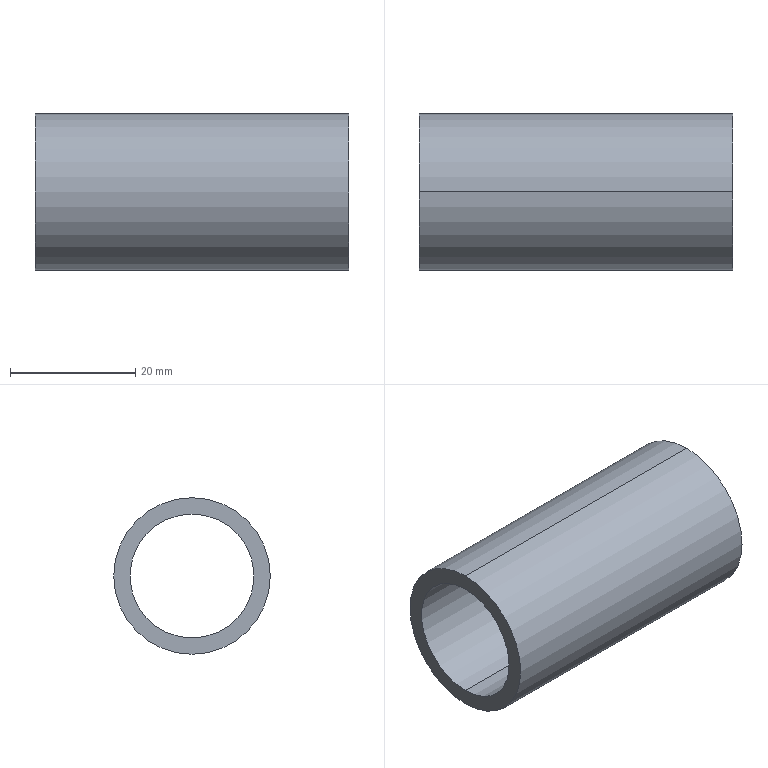Part | STEP file | FUF25-70-A-8 | 1 solid | 6 faces | box 50 x 25 x 25 mm | volume 9148 mm3 | cylinder 4 | plane 2 | commonest cylinder face diameters 19.8 x2 25 x2
STEP:
#1=CARTESIAN_POINT('',(0.,0.,0.));
#2=DIRECTION('',(0.,0.,1.));
#3=DIRECTION('',(1.,0.,0.));
#4=AXIS2_PLACEMENT_3D('',#1,#2,#3);
#5=CARTESIAN_POINT('',(50.,0.,9.9));
#6=VERTEX_POINT('',#5);
#7=CARTESIAN_POINT('',(0.,0.,9.9));
#8=VERTEX_POINT('',#7);
#9=CARTESIAN_POINT('',(50.,0.,9.9));
#10=DIRECTION('',(-1.,0.,0.));
#11=VECTOR('',#10,1.);
#12=LINE('',#9,#11);
#13=CARTESIAN_POINT('',(50.,0.,0.));
#14=DIRECTION('',(-1.,0.,0.));
#15=DIRECTION('',(0.,0.,1.));
#16=AXIS2_PLACEMENT_3D('',#13,#14,#15);
#17=CYLINDRICAL_SURFACE('',#16,9.9);
#18=CARTESIAN_POINT('',(6.283,0.));
#19=DIRECTION('',(0.,1.));
#20=VECTOR('',#19,1.);
#21=LINE('',#18,#20);
#22=(GEOMETRIC_REPRESENTATION_CONTEXT(2)PARAMETRIC_REPRESENTATION_CONTEXT()REPRESENTATION_CONTEXT('',''));
#23=DEFINITIONAL_REPRESENTATION('',(#21),#22);
#24=PCURVE('',#17,#23);
#25=CARTESIAN_POINT('',(50.,0.,0.));
#26=DIRECTION('',(-1.,0.,0.));
#27=DIRECTION('',(0.,0.,1.));
#28=AXIS2_PLACEMENT_3D('',#25,#26,#27);
#29=CYLINDRICAL_SURFACE('',#28,9.9);
#30=CARTESIAN_POINT('',(0.,0.));
#31=DIRECTION('',(0.,1.));
#32=VECTOR('',#31,1.);
#33=LINE('',#30,#32);
#34=(GEOMETRIC_REPRESENTATION_CONTEXT(2)PARAMETRIC_REPRESENTATION_CONTEXT()REPRESENTATION_CONTEXT('',''));
#35=DEFINITIONAL_REPRESENTATION('',(#33),#34);
#36=PCURVE('',#29,#35);
#37=SURFACE_CURVE('',#12,(#24,#36),.PCURVE_S1.);
#38=EDGE_CURVE('',#6,#8,#37,.T.);
#39=ORIENTED_EDGE('',*,*,#38,.T.);
#40=CARTESIAN_POINT('',(0.,0.,-9.9));
#41=VERTEX_POINT('',#40);
#42=CARTESIAN_POINT('',(0.,0.,0.));
#43=DIRECTION('',(1.,0.,0.));
#44=DIRECTION('',(0.,0.,-1.));
#45=AXIS2_PLACEMENT_3D('',#42,#43,#44);
#46=CIRCLE('',#45,9.9);
#47=CARTESIAN_POINT('',(9.425,50.));
#48=DIRECTION('',(-1.,0.));
#49=VECTOR('',#48,1.);
#50=LINE('',#47,#49);
#51=(GEOMETRIC_REPRESENTATION_CONTEXT(2)PARAMETRIC_REPRESENTATION_CONTEXT()REPRESENTATION_CONTEXT('',''));
#52=DEFINITIONAL_REPRESENTATION('',(#50),#51);
#53=PCURVE('',#17,#52);
#54=CARTESIAN_POINT('',(0.,0.,0.));
#55=DIRECTION('',(-1.,0.,0.));
#56=DIRECTION('',(0.,0.,1.));
#57=AXIS2_PLACEMENT_3D('',#54,#55,#56);
#58=PLANE('',#57);
#59=CARTESIAN_POINT('',(-9.9,0.));
#60=CARTESIAN_POINT('',(-9.9,17.147));
#61=CARTESIAN_POINT('',(4.95,8.574));
#62=CARTESIAN_POINT('',(19.8,0.));
#63=CARTESIAN_POINT('',(4.95,-8.574));
#64=CARTESIAN_POINT('',(-9.9,-17.147));
#65=CARTESIAN_POINT('',(-9.9,0.));
#66=(BOUNDED_CURVE()B_SPLINE_CURVE(2,(#59,#60,#61,#62,#63,#64,#65),.UNSPECIFIED.,.T.,.F.)B_SPLINE_CURVE_WITH_KNOTS((1,2,2,2,2,1),(-2.094,0.,2.094,4.189,6.283,8.378),.UNSPECIFIED.)CURVE()GEOMETRIC_REPRESENTATION_ITEM()RATIONAL_B_SPLINE_CURVE((1.,0.5,1.,0.5,1.,0.5,1.))REPRESENTATION_ITEM(''));
#67=(GEOMETRIC_REPRESENTATION_CONTEXT(2)PARAMETRIC_REPRESENTATION_CONTEXT()REPRESENTATION_CONTEXT('',''));
#68=DEFINITIONAL_REPRESENTATION('',(#66),#67);
#69=PCURVE('',#58,#68);
#70=SURFACE_CURVE('',#46,(#53,#69),.PCURVE_S1.);
#71=EDGE_CURVE('',#8,#41,#70,.T.);
#72=ORIENTED_EDGE('',*,*,#71,.T.);
#73=CARTESIAN_POINT('',(50.,0.,-9.9));
#74=VERTEX_POINT('',#73);
#75=CARTESIAN_POINT('',(50.,0.,-9.9));
#76=DIRECTION('',(-1.,0.,0.));
#77=VECTOR('',#76,1.);
#78=LINE('',#75,#77);
#79=CARTESIAN_POINT('',(3.142,0.));
#80=DIRECTION('',(0.,1.));
#81=VECTOR('',#80,1.);
#82=LINE('',#79,#81);
#83=(GEOMETRIC_REPRESENTATION_CONTEXT(2)PARAMETRIC_REPRESENTATION_CONTEXT()REPRESENTATION_CONTEXT('',''));
#84=DEFINITIONAL_REPRESENTATION('',(#82),#83);
#85=PCURVE('',#17,#84);
#86=CARTESIAN_POINT('',(3.142,0.));
#87=DIRECTION('',(0.,1.));
#88=VECTOR('',#87,1.);
#89=LINE('',#86,#88);
#90=(GEOMETRIC_REPRESENTATION_CONTEXT(2)PARAMETRIC_REPRESENTATION_CONTEXT()REPRESENTATION_CONTEXT('',''));
#91=DEFINITIONAL_REPRESENTATION('',(#89),#90);
#92=PCURVE('',#29,#91);
#93=SURFACE_CURVE('',#78,(#85,#92),.PCURVE_S1.);
#94=EDGE_CURVE('',#74,#41,#93,.T.);
#95=ORIENTED_EDGE('',*,*,#94,.F.);
#96=CARTESIAN_POINT('',(50.,0.,0.));
#97=DIRECTION('',(-1.,0.,0.));
#98=DIRECTION('',(0.,0.,1.));
#99=AXIS2_PLACEMENT_3D('',#96,#97,#98);
#100=CIRCLE('',#99,9.9);
#101=CARTESIAN_POINT('',(0.,0.));
#102=DIRECTION('',(1.,0.));
#103=VECTOR('',#102,1.);
#104=LINE('',#101,#103);
#105=(GEOMETRIC_REPRESENTATION_CONTEXT(2)PARAMETRIC_REPRESENTATION_CONTEXT()REPRESENTATION_CONTEXT('',''));
#106=DEFINITIONAL_REPRESENTATION('',(#104),#105);
#107=PCURVE('',#17,#106);
#108=CARTESIAN_POINT('',(50.,0.,0.));
#109=DIRECTION('',(1.,0.,0.));
#110=DIRECTION('',(0.,0.,-1.));
#111=AXIS2_PLACEMENT_3D('',#108,#109,#110);
#112=PLANE('',#111);
#113=CARTESIAN_POINT('',(-9.9,0.));
#114=CARTESIAN_POINT('',(-9.9,17.147));
#115=CARTESIAN_POINT('',(4.95,8.574));
#116=CARTESIAN_POINT('',(19.8,0.));
#117=CARTESIAN_POINT('',(4.95,-8.574));
#118=CARTESIAN_POINT('',(-9.9,-17.147));
#119=CARTESIAN_POINT('',(-9.9,0.));
#120=(BOUNDED_CURVE()B_SPLINE_CURVE(2,(#113,#114,#115,#116,#117,#118,#119),.UNSPECIFIED.,.T.,.F.)B_SPLINE_CURVE_WITH_KNOTS((1,2,2,2,2,1),(-2.094,0.,2.094,4.189,6.283,8.378),.UNSPECIFIED.)CURVE()GEOMETRIC_REPRESENTATION_ITEM()RATIONAL_B_SPLINE_CURVE((1.,0.5,1.,0.5,1.,0.5,1.))REPRESENTATION_ITEM(''));
#121=(GEOMETRIC_REPRESENTATION_CONTEXT(2)PARAMETRIC_REPRESENTATION_CONTEXT()REPRESENTATION_CONTEXT('',''));
#122=DEFINITIONAL_REPRESENTATION('',(#120),#121);
#123=PCURVE('',#112,#122);
#124=SURFACE_CURVE('',#100,(#107,#123),.PCURVE_S1.);
#125=EDGE_CURVE('',#74,#6,#124,.T.);
#126=ORIENTED_EDGE('',*,*,#125,.T.);
#127=EDGE_LOOP('',(#39,#72,#95,#126));
#128=FACE_BOUND('',#127,.F.);
#129=ADVANCED_FACE('',(#128),#17,.F.);
#130=CARTESIAN_POINT('',(0.,0.,-12.5));
#131=VERTEX_POINT('',#130);
#132=CARTESIAN_POINT('',(0.,0.,12.5));
#133=VERTEX_POINT('',#132);
#134=CARTESIAN_POINT('',(0.,0.,0.));
#135=DIRECTION('',(1.,0.,0.));
#136=DIRECTION('',(0.,0.,-1.));
#137=AXIS2_PLACEMENT_3D('',#134,#135,#136);
#138=CIRCLE('',#137,12.5);
#139=CARTESIAN_POINT('',(0.,0.,0.));
#140=DIRECTION('',(1.,0.,0.));
#141=DIRECTION('',(0.,0.,-1.));
#142=AXIS2_PLACEMENT_3D('',#139,#140,#141);
#143=CYLINDRICAL_SURFACE('',#142,12.5);
#144=CARTESIAN_POINT('',(0.,0.));
#145=DIRECTION('',(1.,0.));
#146=VECTOR('',#145,1.);
#147=LINE('',#144,#146);
#148=(GEOMETRIC_REPRESENTATION_CONTEXT(2)PARAMETRIC_REPRESENTATION_CONTEXT()REPRESENTATION_CONTEXT('',''));
#149=DEFINITIONAL_REPRESENTATION('',(#147),#148);
#150=PCURVE('',#143,#149);
#151=CARTESIAN_POINT('',(-12.5,0.));
#152=CARTESIAN_POINT('',(-12.5,21.651));
#153=CARTESIAN_POINT('',(6.25,10.825));
#154=CARTESIAN_POINT('',(25.,0.));
#155=CARTESIAN_POINT('',(6.25,-10.825));
#156=CARTESIAN_POINT('',(-12.5,-21.651));
#157=CARTESIAN_POINT('',(-12.5,0.));
#158=(BOUNDED_CURVE()B_SPLINE_CURVE(2,(#151,#152,#153,#154,#155,#156,#157),.UNSPECIFIED.,.T.,.F.)B_SPLINE_CURVE_WITH_KNOTS((1,2,2,2,2,1),(-2.094,0.,2.094,4.189,6.283,8.378),.UNSPECIFIED.)CURVE()GEOMETRIC_REPRESENTATION_ITEM()RATIONAL_B_SPLINE_CURVE((1.,0.5,1.,0.5,1.,0.5,1.))REPRESENTATION_ITEM(''));
#159=(GEOMETRIC_REPRESENTATION_CONTEXT(2)PARAMETRIC_REPRESENTATION_CONTEXT()REPRESENTATION_CONTEXT('',''));
#160=DEFINITIONAL_REPRESENTATION('',(#158),#159);
#161=PCURVE('',#58,#160);
#162=SURFACE_CURVE('',#138,(#150,#161),.PCURVE_S1.);
#163=EDGE_CURVE('',#131,#133,#162,.T.);
#164=ORIENTED_EDGE('',*,*,#163,.T.);
#165=CARTESIAN_POINT('',(50.,0.,12.5));
#166=VERTEX_POINT('',#165);
#167=CARTESIAN_POINT('',(0.,0.,12.5));
#168=DIRECTION('',(1.,0.,0.));
#169=VECTOR('',#168,1.);
#170=LINE('',#167,#169);
#171=CARTESIAN_POINT('',(3.142,0.));
#172=DIRECTION('',(0.,1.));
#173=VECTOR('',#172,1.);
#174=LINE('',#171,#173);
#175=(GEOMETRIC_REPRESENTATION_CONTEXT(2)PARAMETRIC_REPRESENTATION_CONTEXT()REPRESENTATION_CONTEXT('',''));
#176=DEFINITIONAL_REPRESENTATION('',(#174),#175);
#177=PCURVE('',#143,#176);
#178=CARTESIAN_POINT('',(0.,0.,0.));
#179=DIRECTION('',(1.,0.,0.));
#180=DIRECTION('',(0.,0.,-1.));
#181=AXIS2_PLACEMENT_3D('',#178,#179,#180);
#182=CYLINDRICAL_SURFACE('',#181,12.5);
#183=CARTESIAN_POINT('',(3.142,0.));
#184=DIRECTION('',(0.,1.));
#185=VECTOR('',#184,1.);
#186=LINE('',#183,#185);
#187=(GEOMETRIC_REPRESENTATION_CONTEXT(2)PARAMETRIC_REPRESENTATION_CONTEXT()REPRESENTATION_CONTEXT('',''));
#188=DEFINITIONAL_REPRESENTATION('',(#186),#187);
#189=PCURVE('',#182,#188);
#190=SURFACE_CURVE('',#170,(#177,#189),.PCURVE_S1.);
#191=EDGE_CURVE('',#133,#166,#190,.T.);
#192=ORIENTED_EDGE('',*,*,#191,.T.);
#193=CARTESIAN_POINT('',(50.,0.,-12.5));
#194=VERTEX_POINT('',#193);
#195=CARTESIAN_POINT('',(50.,0.,0.));
#196=DIRECTION('',(-1.,0.,0.));
#197=DIRECTION('',(0.,0.,1.));
#198=AXIS2_PLACEMENT_3D('',#195,#196,#197);
#199=CIRCLE('',#198,12.5);
#200=CARTESIAN_POINT('',(3.142,50.));
#201=DIRECTION('',(-1.,0.));
#202=VECTOR('',#201,1.);
#203=LINE('',#200,#202);
#204=(GEOMETRIC_REPRESENTATION_CONTEXT(2)PARAMETRIC_REPRESENTATION_CONTEXT()REPRESENTATION_CONTEXT('',''));
#205=DEFINITIONAL_REPRESENTATION('',(#203),#204);
#206=PCURVE('',#143,#205);
#207=CARTESIAN_POINT('',(-12.5,0.));
#208=CARTESIAN_POINT('',(-12.5,21.651));
#209=CARTESIAN_POINT('',(6.25,10.825));
#210=CARTESIAN_POINT('',(25.,0.));
#211=CARTESIAN_POINT('',(6.25,-10.825));
#212=CARTESIAN_POINT('',(-12.5,-21.651));
#213=CARTESIAN_POINT('',(-12.5,0.));
#214=(BOUNDED_CURVE()B_SPLINE_CURVE(2,(#207,#208,#209,#210,#211,#212,#213),.UNSPECIFIED.,.T.,.F.)B_SPLINE_CURVE_WITH_KNOTS((1,2,2,2,2,1),(-2.094,0.,2.094,4.189,6.283,8.378),.UNSPECIFIED.)CURVE()GEOMETRIC_REPRESENTATION_ITEM()RATIONAL_B_SPLINE_CURVE((1.,0.5,1.,0.5,1.,0.5,1.))REPRESENTATION_ITEM(''));
#215=(GEOMETRIC_REPRESENTATION_CONTEXT(2)PARAMETRIC_REPRESENTATION_CONTEXT()REPRESENTATION_CONTEXT('',''));
#216=DEFINITIONAL_REPRESENTATION('',(#214),#215);
#217=PCURVE('',#112,#216);
#218=SURFACE_CURVE('',#199,(#206,#217),.PCURVE_S1.);
#219=EDGE_CURVE('',#166,#194,#218,.T.);
#220=ORIENTED_EDGE('',*,*,#219,.T.);
#221=CARTESIAN_POINT('',(0.,0.,-12.5));
#222=DIRECTION('',(1.,0.,0.));
#223=VECTOR('',#222,1.);
#224=LINE('',#221,#223);
#225=CARTESIAN_POINT('',(0.,0.));
#226=DIRECTION('',(0.,1.));
#227=VECTOR('',#226,1.);
#228=LINE('',#225,#227);
#229=(GEOMETRIC_REPRESENTATION_CONTEXT(2)PARAMETRIC_REPRESENTATION_CONTEXT()REPRESENTATION_CONTEXT('',''));
#230=DEFINITIONAL_REPRESENTATION('',(#228),#229);
#231=PCURVE('',#143,#230);
#232=CARTESIAN_POINT('',(6.283,0.));
#233=DIRECTION('',(0.,1.));
#234=VECTOR('',#233,1.);
#235=LINE('',#232,#234);
#236=(GEOMETRIC_REPRESENTATION_CONTEXT(2)PARAMETRIC_REPRESENTATION_CONTEXT()REPRESENTATION_CONTEXT('',''));
#237=DEFINITIONAL_REPRESENTATION('',(#235),#236);
#238=PCURVE('',#182,#237);
#239=SURFACE_CURVE('',#224,(#231,#238),.PCURVE_S1.);
#240=EDGE_CURVE('',#131,#194,#239,.T.);
#241=ORIENTED_EDGE('',*,*,#240,.F.);
#242=EDGE_LOOP('',(#164,#192,#220,#241));
#243=FACE_BOUND('',#242,.T.);
#244=ADVANCED_FACE('',(#243),#143,.T.);
#245=CARTESIAN_POINT('',(50.,0.,0.));
#246=DIRECTION('',(-1.,0.,0.));
#247=DIRECTION('',(0.,0.,1.));
#248=AXIS2_PLACEMENT_3D('',#245,#246,#247);
#249=CIRCLE('',#248,9.9);
#250=CARTESIAN_POINT('',(-9.9,0.));
#251=CARTESIAN_POINT('',(-9.9,17.147));
#252=CARTESIAN_POINT('',(4.95,8.574));
#253=CARTESIAN_POINT('',(19.8,0.));
#254=CARTESIAN_POINT('',(4.95,-8.574));
#255=CARTESIAN_POINT('',(-9.9,-17.147));
#256=CARTESIAN_POINT('',(-9.9,0.));
#257=(BOUNDED_CURVE()B_SPLINE_CURVE(2,(#250,#251,#252,#253,#254,#255,#256),.UNSPECIFIED.,.T.,.F.)B_SPLINE_CURVE_WITH_KNOTS((1,2,2,2,2,1),(-2.094,0.,2.094,4.189,6.283,8.378),.UNSPECIFIED.)CURVE()GEOMETRIC_REPRESENTATION_ITEM()RATIONAL_B_SPLINE_CURVE((1.,0.5,1.,0.5,1.,0.5,1.))REPRESENTATION_ITEM(''));
#258=(GEOMETRIC_REPRESENTATION_CONTEXT(2)PARAMETRIC_REPRESENTATION_CONTEXT()REPRESENTATION_CONTEXT('',''));
#259=DEFINITIONAL_REPRESENTATION('',(#257),#258);
#260=PCURVE('',#112,#259);
#261=CARTESIAN_POINT('',(0.,0.));
#262=DIRECTION('',(1.,0.));
#263=VECTOR('',#262,1.);
#264=LINE('',#261,#263);
#265=(GEOMETRIC_REPRESENTATION_CONTEXT(2)PARAMETRIC_REPRESENTATION_CONTEXT()REPRESENTATION_CONTEXT('',''));
#266=DEFINITIONAL_REPRESENTATION('',(#264),#265);
#267=PCURVE('',#29,#266);
#268=SURFACE_CURVE('',#249,(#260,#267),.PCURVE_S1.);
#269=EDGE_CURVE('',#6,#74,#268,.T.);
#270=ORIENTED_EDGE('',*,*,#269,.T.);
#271=ORIENTED_EDGE('',*,*,#125,.T.);
#272=EDGE_LOOP('',(#270,#271));
#273=FACE_BOUND('',#272,.T.);
#274=CARTESIAN_POINT('',(50.,0.,0.));
#275=DIRECTION('',(-1.,0.,0.));
#276=DIRECTION('',(0.,0.,1.));
#277=AXIS2_PLACEMENT_3D('',#274,#275,#276);
#278=CIRCLE('',#277,12.5);
#279=CARTESIAN_POINT('',(-12.5,0.));
#280=CARTESIAN_POINT('',(-12.5,21.651));
#281=CARTESIAN_POINT('',(6.25,10.825));
#282=CARTESIAN_POINT('',(25.,0.));
#283=CARTESIAN_POINT('',(6.25,-10.825));
#284=CARTESIAN_POINT('',(-12.5,-21.651));
#285=CARTESIAN_POINT('',(-12.5,0.));
#286=(BOUNDED_CURVE()B_SPLINE_CURVE(2,(#279,#280,#281,#282,#283,#284,#285),.UNSPECIFIED.,.T.,.F.)B_SPLINE_CURVE_WITH_KNOTS((1,2,2,2,2,1),(-2.094,0.,2.094,4.189,6.283,8.378),.UNSPECIFIED.)CURVE()GEOMETRIC_REPRESENTATION_ITEM()RATIONAL_B_SPLINE_CURVE((1.,0.5,1.,0.5,1.,0.5,1.))REPRESENTATION_ITEM(''));
#287=(GEOMETRIC_REPRESENTATION_CONTEXT(2)PARAMETRIC_REPRESENTATION_CONTEXT()REPRESENTATION_CONTEXT('',''));
#288=DEFINITIONAL_REPRESENTATION('',(#286),#287);
#289=PCURVE('',#112,#288);
#290=CARTESIAN_POINT('',(9.425,50.));
#291=DIRECTION('',(-1.,0.));
#292=VECTOR('',#291,1.);
#293=LINE('',#290,#292);
#294=(GEOMETRIC_REPRESENTATION_CONTEXT(2)PARAMETRIC_REPRESENTATION_CONTEXT()REPRESENTATION_CONTEXT('',''));
#295=DEFINITIONAL_REPRESENTATION('',(#293),#294);
#296=PCURVE('',#182,#295);
#297=SURFACE_CURVE('',#278,(#289,#296),.PCURVE_S1.);
#298=EDGE_CURVE('',#194,#166,#297,.T.);
#299=ORIENTED_EDGE('',*,*,#298,.F.);
#300=ORIENTED_EDGE('',*,*,#219,.F.);
#301=EDGE_LOOP('',(#299,#300));
#302=FACE_BOUND('',#301,.T.);
#303=ADVANCED_FACE('',(#273,#302),#112,.T.);
#304=ORIENTED_EDGE('',*,*,#71,.T.);
#305=CARTESIAN_POINT('',(0.,0.,0.));
#306=DIRECTION('',(1.,0.,0.));
#307=DIRECTION('',(0.,0.,-1.));
#308=AXIS2_PLACEMENT_3D('',#305,#306,#307);
#309=CIRCLE('',#308,9.9);
#310=CARTESIAN_POINT('',(-9.9,0.));
#311=CARTESIAN_POINT('',(-9.9,17.147));
#312=CARTESIAN_POINT('',(4.95,8.574));
#313=CARTESIAN_POINT('',(19.8,0.));
#314=CARTESIAN_POINT('',(4.95,-8.574));
#315=CARTESIAN_POINT('',(-9.9,-17.147));
#316=CARTESIAN_POINT('',(-9.9,0.));
#317=(BOUNDED_CURVE()B_SPLINE_CURVE(2,(#310,#311,#312,#313,#314,#315,#316),.UNSPECIFIED.,.T.,.F.)B_SPLINE_CURVE_WITH_KNOTS((1,2,2,2,2,1),(-2.094,0.,2.094,4.189,6.283,8.378),.UNSPECIFIED.)CURVE()GEOMETRIC_REPRESENTATION_ITEM()RATIONAL_B_SPLINE_CURVE((1.,0.5,1.,0.5,1.,0.5,1.))REPRESENTATION_ITEM(''));
#318=(GEOMETRIC_REPRESENTATION_CONTEXT(2)PARAMETRIC_REPRESENTATION_CONTEXT()REPRESENTATION_CONTEXT('',''));
#319=DEFINITIONAL_REPRESENTATION('',(#317),#318);
#320=PCURVE('',#58,#319);
#321=CARTESIAN_POINT('',(3.142,50.));
#322=DIRECTION('',(-1.,0.));
#323=VECTOR('',#322,1.);
#324=LINE('',#321,#323);
#325=(GEOMETRIC_REPRESENTATION_CONTEXT(2)PARAMETRIC_REPRESENTATION_CONTEXT()REPRESENTATION_CONTEXT('',''));
#326=DEFINITIONAL_REPRESENTATION('',(#324),#325);
#327=PCURVE('',#29,#326);
#328=SURFACE_CURVE('',#309,(#320,#327),.PCURVE_S1.);
#329=EDGE_CURVE('',#41,#8,#328,.T.);
#330=ORIENTED_EDGE('',*,*,#329,.T.);
#331=EDGE_LOOP('',(#304,#330));
#332=FACE_BOUND('',#331,.T.);
#333=ORIENTED_EDGE('',*,*,#163,.F.);
#334=CARTESIAN_POINT('',(0.,0.,0.));
#335=DIRECTION('',(1.,0.,0.));
#336=DIRECTION('',(0.,0.,-1.));
#337=AXIS2_PLACEMENT_3D('',#334,#335,#336);
#338=CIRCLE('',#337,12.5);
#339=CARTESIAN_POINT('',(-12.5,0.));
#340=CARTESIAN_POINT('',(-12.5,21.651));
#341=CARTESIAN_POINT('',(6.25,10.825));
#342=CARTESIAN_POINT('',(25.,0.));
#343=CARTESIAN_POINT('',(6.25,-10.825));
#344=CARTESIAN_POINT('',(-12.5,-21.651));
#345=CARTESIAN_POINT('',(-12.5,0.));
#346=(BOUNDED_CURVE()B_SPLINE_CURVE(2,(#339,#340,#341,#342,#343,#344,#345),.UNSPECIFIED.,.T.,.F.)B_SPLINE_CURVE_WITH_KNOTS((1,2,2,2,2,1),(-2.094,0.,2.094,4.189,6.283,8.378),.UNSPECIFIED.)CURVE()GEOMETRIC_REPRESENTATION_ITEM()RATIONAL_B_SPLINE_CURVE((1.,0.5,1.,0.5,1.,0.5,1.))REPRESENTATION_ITEM(''));
#347=(GEOMETRIC_REPRESENTATION_CONTEXT(2)PARAMETRIC_REPRESENTATION_CONTEXT()REPRESENTATION_CONTEXT('',''));
#348=DEFINITIONAL_REPRESENTATION('',(#346),#347);
#349=PCURVE('',#58,#348);
#350=CARTESIAN_POINT('',(0.,0.));
#351=DIRECTION('',(1.,0.));
#352=VECTOR('',#351,1.);
#353=LINE('',#350,#352);
#354=(GEOMETRIC_REPRESENTATION_CONTEXT(2)PARAMETRIC_REPRESENTATION_CONTEXT()REPRESENTATION_CONTEXT('',''));
#355=DEFINITIONAL_REPRESENTATION('',(#353),#354);
#356=PCURVE('',#182,#355);
#357=SURFACE_CURVE('',#338,(#349,#356),.PCURVE_S1.);
#358=EDGE_CURVE('',#133,#131,#357,.T.);
#359=ORIENTED_EDGE('',*,*,#358,.F.);
#360=EDGE_LOOP('',(#333,#359));
#361=FACE_BOUND('',#360,.T.);
#362=ADVANCED_FACE('',(#332,#361),#58,.T.);
#363=ORIENTED_EDGE('',*,*,#191,.F.);
#364=ORIENTED_EDGE('',*,*,#358,.T.);
#365=ORIENTED_EDGE('',*,*,#240,.T.);
#366=ORIENTED_EDGE('',*,*,#298,.T.);
#367=EDGE_LOOP('',(#363,#364,#365,#366));
#368=FACE_BOUND('',#367,.T.);
#369=ADVANCED_FACE('',(#368),#182,.T.);
#370=ORIENTED_EDGE('',*,*,#329,.T.);
#371=ORIENTED_EDGE('',*,*,#38,.F.);
#372=ORIENTED_EDGE('',*,*,#269,.T.);
#373=ORIENTED_EDGE('',*,*,#94,.T.);
#374=EDGE_LOOP('',(#370,#371,#372,#373));
#375=FACE_BOUND('',#374,.F.);
#376=ADVANCED_FACE('',(#375),#29,.F.);
#377=CLOSED_SHELL('',(#129,#244,#303,#362,#369,#376));
#378=MANIFOLD_SOLID_BREP('',#377);
#379=(LENGTH_UNIT()NAMED_UNIT(*)SI_UNIT(.MILLI.,.METRE.));
#380=UNCERTAINTY_MEASURE_WITH_UNIT(LENGTH_MEASURE(0.0000001),#379,'','');
#381=(NAMED_UNIT(*)PLANE_ANGLE_UNIT()SI_UNIT($,.RADIAN.));
#382=(NAMED_UNIT(*)SI_UNIT($,.STERADIAN.)SOLID_ANGLE_UNIT());
#383=(GEOMETRIC_REPRESENTATION_CONTEXT(3)GLOBAL_UNCERTAINTY_ASSIGNED_CONTEXT((#380))GLOBAL_UNIT_ASSIGNED_CONTEXT((#379,#381,#382))REPRESENTATION_CONTEXT('',''));
#384=ADVANCED_BREP_SHAPE_REPRESENTATION('',(#4,#378),#383);